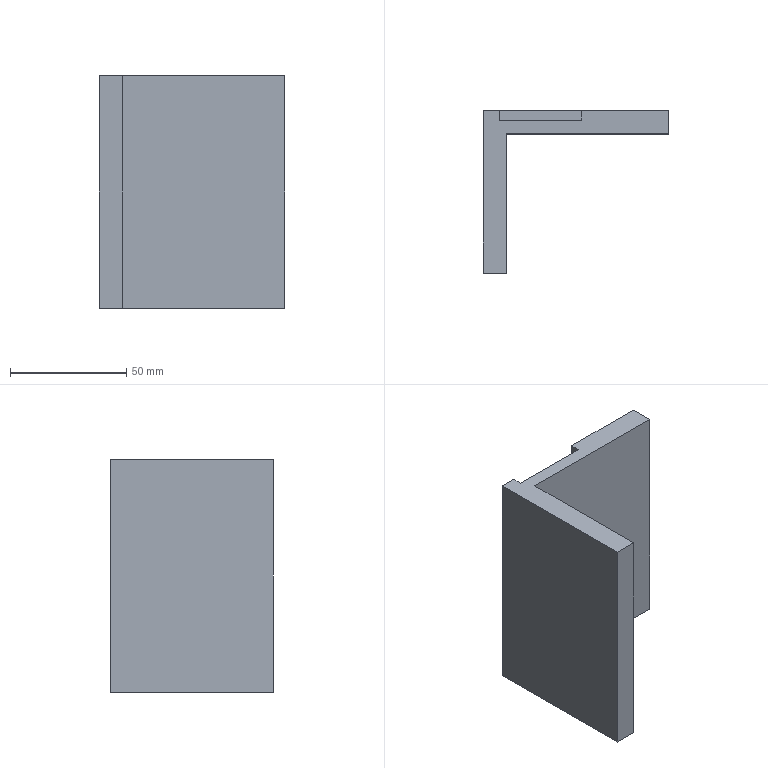Part | SolidWorks | features Cut 1, Extrusion 1 | 1 solid | 12 faces | box 80 x 70 x 100 mm | volume 131100 mm3 | plane 12
STEP:
#1=CARTESIAN_POINT('',(-37.5,32.788,0.));
#2=VERTEX_POINT('',#1);
#3=CARTESIAN_POINT('',(-37.5,-37.212,0.));
#4=VERTEX_POINT('',#3);
#5=CARTESIAN_POINT('',(-37.5,-37.212,0.));
#6=DIRECTION('',(0.,-1.,0.));
#7=VECTOR('',#6,1000.);
#8=LINE('',#5,#7);
#9=EDGE_CURVE('',#2,#4,#8,.T.);
#10=ORIENTED_EDGE('',*,*,#9,.T.);
#11=CARTESIAN_POINT('',(-37.5,-37.212,100.));
#12=VERTEX_POINT('',#11);
#13=CARTESIAN_POINT('',(-37.5,-37.212,100.));
#14=DIRECTION('',(0.,0.,-1.));
#15=VECTOR('',#14,1000.);
#16=LINE('',#13,#15);
#17=EDGE_CURVE('',#12,#4,#16,.T.);
#18=ORIENTED_EDGE('',*,*,#17,.F.);
#19=CARTESIAN_POINT('',(-37.5,32.788,100.));
#20=VERTEX_POINT('',#19);
#21=CARTESIAN_POINT('',(-37.5,-37.212,100.));
#22=DIRECTION('',(0.,-1.,0.));
#23=VECTOR('',#22,1000.);
#24=LINE('',#21,#23);
#25=EDGE_CURVE('',#20,#12,#24,.T.);
#26=ORIENTED_EDGE('',*,*,#25,.F.);
#27=CARTESIAN_POINT('',(-37.5,32.788,100.));
#28=DIRECTION('',(0.,0.,-1.));
#29=VECTOR('',#28,1000.);
#30=LINE('',#27,#29);
#31=EDGE_CURVE('',#20,#2,#30,.T.);
#32=ORIENTED_EDGE('',*,*,#31,.T.);
#33=EDGE_LOOP('',(#10,#18,#26,#32));
#34=FACE_OUTER_BOUND('',#33,.T.);
#35=CARTESIAN_POINT('',(-37.5,-37.212,100.));
#36=DIRECTION('',(1.,0.,0.));
#37=DIRECTION('',(0.,0.,-1.));
#38=AXIS2_PLACEMENT_3D('',#35,#36,#37);
#39=PLANE('',#38);
#40=ADVANCED_FACE('',(#34),#39,.F.);
#41=CARTESIAN_POINT('',(-27.5,-37.212,0.));
#42=VERTEX_POINT('',#41);
#43=CARTESIAN_POINT('',(-27.5,-37.212,0.));
#44=DIRECTION('',(1.,0.,0.));
#45=VECTOR('',#44,1000.);
#46=LINE('',#43,#45);
#47=EDGE_CURVE('',#4,#42,#46,.T.);
#48=ORIENTED_EDGE('',*,*,#47,.T.);
#49=CARTESIAN_POINT('',(-27.5,-37.212,100.));
#50=VERTEX_POINT('',#49);
#51=CARTESIAN_POINT('',(-27.5,-37.212,100.));
#52=DIRECTION('',(0.,0.,-1.));
#53=VECTOR('',#52,1000.);
#54=LINE('',#51,#53);
#55=EDGE_CURVE('',#50,#42,#54,.T.);
#56=ORIENTED_EDGE('',*,*,#55,.F.);
#57=CARTESIAN_POINT('',(-27.5,-37.212,100.));
#58=DIRECTION('',(1.,0.,0.));
#59=VECTOR('',#58,1000.);
#60=LINE('',#57,#59);
#61=EDGE_CURVE('',#12,#50,#60,.T.);
#62=ORIENTED_EDGE('',*,*,#61,.F.);
#63=ORIENTED_EDGE('',*,*,#17,.T.);
#64=EDGE_LOOP('',(#48,#56,#62,#63));
#65=FACE_OUTER_BOUND('',#64,.T.);
#66=CARTESIAN_POINT('',(-27.5,-37.212,100.));
#67=DIRECTION('',(0.,1.,0.));
#68=DIRECTION('',(0.,0.,1.));
#69=AXIS2_PLACEMENT_3D('',#66,#67,#68);
#70=PLANE('',#69);
#71=ADVANCED_FACE('',(#65),#70,.F.);
#72=CARTESIAN_POINT('',(-27.5,22.788,0.));
#73=VERTEX_POINT('',#72);
#74=CARTESIAN_POINT('',(-27.5,22.788,0.));
#75=DIRECTION('',(0.,1.,0.));
#76=VECTOR('',#75,1000.);
#77=LINE('',#74,#76);
#78=EDGE_CURVE('',#42,#73,#77,.T.);
#79=ORIENTED_EDGE('',*,*,#78,.T.);
#80=CARTESIAN_POINT('',(-27.5,22.788,100.));
#81=VERTEX_POINT('',#80);
#82=CARTESIAN_POINT('',(-27.5,22.788,100.));
#83=DIRECTION('',(0.,0.,-1.));
#84=VECTOR('',#83,1000.);
#85=LINE('',#82,#84);
#86=EDGE_CURVE('',#81,#73,#85,.T.);
#87=ORIENTED_EDGE('',*,*,#86,.F.);
#88=CARTESIAN_POINT('',(-27.5,22.788,100.));
#89=DIRECTION('',(0.,1.,0.));
#90=VECTOR('',#89,1000.);
#91=LINE('',#88,#90);
#92=EDGE_CURVE('',#50,#81,#91,.T.);
#93=ORIENTED_EDGE('',*,*,#92,.F.);
#94=ORIENTED_EDGE('',*,*,#55,.T.);
#95=EDGE_LOOP('',(#79,#87,#93,#94));
#96=FACE_OUTER_BOUND('',#95,.T.);
#97=CARTESIAN_POINT('',(-27.5,22.788,100.));
#98=DIRECTION('',(-1.,0.,0.));
#99=DIRECTION('',(0.,-1.,0.));
#100=AXIS2_PLACEMENT_3D('',#97,#98,#99);
#101=PLANE('',#100);
#102=ADVANCED_FACE('',(#96),#101,.F.);
#103=CARTESIAN_POINT('',(42.5,22.788,0.));
#104=VERTEX_POINT('',#103);
#105=CARTESIAN_POINT('',(42.5,22.788,0.));
#106=DIRECTION('',(1.,0.,0.));
#107=VECTOR('',#106,1000.);
#108=LINE('',#105,#107);
#109=EDGE_CURVE('',#73,#104,#108,.T.);
#110=ORIENTED_EDGE('',*,*,#109,.T.);
#111=CARTESIAN_POINT('',(42.5,22.788,100.));
#112=VERTEX_POINT('',#111);
#113=CARTESIAN_POINT('',(42.5,22.788,100.));
#114=DIRECTION('',(0.,0.,-1.));
#115=VECTOR('',#114,1000.);
#116=LINE('',#113,#115);
#117=EDGE_CURVE('',#112,#104,#116,.T.);
#118=ORIENTED_EDGE('',*,*,#117,.F.);
#119=CARTESIAN_POINT('',(42.5,22.788,100.));
#120=DIRECTION('',(1.,0.,0.));
#121=VECTOR('',#120,1000.);
#122=LINE('',#119,#121);
#123=EDGE_CURVE('',#81,#112,#122,.T.);
#124=ORIENTED_EDGE('',*,*,#123,.F.);
#125=ORIENTED_EDGE('',*,*,#86,.T.);
#126=EDGE_LOOP('',(#110,#118,#124,#125));
#127=FACE_OUTER_BOUND('',#126,.T.);
#128=CARTESIAN_POINT('',(42.5,22.788,100.));
#129=DIRECTION('',(0.,1.,0.));
#130=DIRECTION('',(-1.,0.,0.));
#131=AXIS2_PLACEMENT_3D('',#128,#129,#130);
#132=PLANE('',#131);
#133=ADVANCED_FACE('',(#127),#132,.F.);
#134=CARTESIAN_POINT('',(42.5,32.788,0.));
#135=VERTEX_POINT('',#134);
#136=CARTESIAN_POINT('',(42.5,32.788,0.));
#137=DIRECTION('',(0.,1.,0.));
#138=VECTOR('',#137,1000.);
#139=LINE('',#136,#138);
#140=EDGE_CURVE('',#104,#135,#139,.T.);
#141=ORIENTED_EDGE('',*,*,#140,.T.);
#142=CARTESIAN_POINT('',(42.5,32.788,100.));
#143=VERTEX_POINT('',#142);
#144=CARTESIAN_POINT('',(42.5,32.788,100.));
#145=DIRECTION('',(0.,0.,-1.));
#146=VECTOR('',#145,1000.);
#147=LINE('',#144,#146);
#148=EDGE_CURVE('',#143,#135,#147,.T.);
#149=ORIENTED_EDGE('',*,*,#148,.F.);
#150=CARTESIAN_POINT('',(42.5,32.788,100.));
#151=DIRECTION('',(0.,1.,0.));
#152=VECTOR('',#151,1000.);
#153=LINE('',#150,#152);
#154=EDGE_CURVE('',#112,#143,#153,.T.);
#155=ORIENTED_EDGE('',*,*,#154,.F.);
#156=ORIENTED_EDGE('',*,*,#117,.T.);
#157=EDGE_LOOP('',(#141,#149,#155,#156));
#158=FACE_OUTER_BOUND('',#157,.T.);
#159=CARTESIAN_POINT('',(42.5,32.788,100.));
#160=DIRECTION('',(-1.,0.,0.));
#161=DIRECTION('',(0.,0.,1.));
#162=AXIS2_PLACEMENT_3D('',#159,#160,#161);
#163=PLANE('',#162);
#164=ADVANCED_FACE('',(#158),#163,.F.);
#165=CARTESIAN_POINT('',(4.86,32.788,40.));
#166=VERTEX_POINT('',#165);
#167=CARTESIAN_POINT('',(-30.458,32.788,40.));
#168=VERTEX_POINT('',#167);
#169=CARTESIAN_POINT('',(4.86,32.788,40.));
#170=DIRECTION('',(-1.,0.,0.));
#171=VECTOR('',#170,1000.);
#172=LINE('',#169,#171);
#173=EDGE_CURVE('',#166,#168,#172,.T.);
#174=ORIENTED_EDGE('',*,*,#173,.F.);
#175=CARTESIAN_POINT('',(4.86,32.788,100.));
#176=VERTEX_POINT('',#175);
#177=CARTESIAN_POINT('',(4.86,32.788,40.));
#178=DIRECTION('',(0.,0.,1.));
#179=VECTOR('',#178,1000.);
#180=LINE('',#177,#179);
#181=EDGE_CURVE('',#166,#176,#180,.T.);
#182=ORIENTED_EDGE('',*,*,#181,.T.);
#183=CARTESIAN_POINT('',(-37.5,32.788,100.));
#184=DIRECTION('',(-1.,0.,0.));
#185=VECTOR('',#184,1000.);
#186=LINE('',#183,#185);
#187=EDGE_CURVE('',#143,#176,#186,.T.);
#188=ORIENTED_EDGE('',*,*,#187,.F.);
#189=ORIENTED_EDGE('',*,*,#148,.T.);
#190=CARTESIAN_POINT('',(-37.5,32.788,0.));
#191=DIRECTION('',(-1.,0.,0.));
#192=VECTOR('',#191,1000.);
#193=LINE('',#190,#192);
#194=EDGE_CURVE('',#135,#2,#193,.T.);
#195=ORIENTED_EDGE('',*,*,#194,.T.);
#196=ORIENTED_EDGE('',*,*,#31,.F.);
#197=CARTESIAN_POINT('',(-30.458,32.788,100.));
#198=VERTEX_POINT('',#197);
#199=CARTESIAN_POINT('',(-37.5,32.788,100.));
#200=DIRECTION('',(-1.,0.,0.));
#201=VECTOR('',#200,1000.);
#202=LINE('',#199,#201);
#203=EDGE_CURVE('',#198,#20,#202,.T.);
#204=ORIENTED_EDGE('',*,*,#203,.F.);
#205=CARTESIAN_POINT('',(-30.458,32.788,40.));
#206=DIRECTION('',(0.,0.,1.));
#207=VECTOR('',#206,1000.);
#208=LINE('',#205,#207);
#209=EDGE_CURVE('',#168,#198,#208,.T.);
#210=ORIENTED_EDGE('',*,*,#209,.F.);
#211=EDGE_LOOP('',(#174,#182,#188,#189,#195,#196,#204,#210));
#212=FACE_OUTER_BOUND('',#211,.T.);
#213=CARTESIAN_POINT('',(-37.5,32.788,100.));
#214=DIRECTION('',(0.,-1.,0.));
#215=DIRECTION('',(1.,0.,0.));
#216=AXIS2_PLACEMENT_3D('',#213,#214,#215);
#217=PLANE('',#216);
#218=ADVANCED_FACE('',(#212),#217,.F.);
#219=ORIENTED_EDGE('',*,*,#187,.T.);
#220=CARTESIAN_POINT('',(4.86,28.588,100.));
#221=VERTEX_POINT('',#220);
#222=CARTESIAN_POINT('',(4.86,28.588,100.));
#223=DIRECTION('',(0.,1.,0.));
#224=VECTOR('',#223,1000.);
#225=LINE('',#222,#224);
#226=EDGE_CURVE('',#221,#176,#225,.T.);
#227=ORIENTED_EDGE('',*,*,#226,.F.);
#228=CARTESIAN_POINT('',(-30.458,28.588,100.));
#229=VERTEX_POINT('',#228);
#230=CARTESIAN_POINT('',(-30.458,28.588,100.));
#231=DIRECTION('',(1.,0.,0.));
#232=VECTOR('',#231,1000.);
#233=LINE('',#230,#232);
#234=EDGE_CURVE('',#229,#221,#233,.T.);
#235=ORIENTED_EDGE('',*,*,#234,.F.);
#236=CARTESIAN_POINT('',(-30.458,32.788,100.));
#237=DIRECTION('',(0.,-1.,0.));
#238=VECTOR('',#237,1000.);
#239=LINE('',#236,#238);
#240=EDGE_CURVE('',#198,#229,#239,.T.);
#241=ORIENTED_EDGE('',*,*,#240,.F.);
#242=ORIENTED_EDGE('',*,*,#203,.T.);
#243=ORIENTED_EDGE('',*,*,#25,.T.);
#244=ORIENTED_EDGE('',*,*,#61,.T.);
#245=ORIENTED_EDGE('',*,*,#92,.T.);
#246=ORIENTED_EDGE('',*,*,#123,.T.);
#247=ORIENTED_EDGE('',*,*,#154,.T.);
#248=EDGE_LOOP('',(#219,#227,#235,#241,#242,#243,#244,#245,#246,#247));
#249=FACE_OUTER_BOUND('',#248,.T.);
#250=CARTESIAN_POINT('',(0.,0.,100.));
#251=DIRECTION('',(0.,0.,-1.));
#252=DIRECTION('',(-1.,0.,0.));
#253=AXIS2_PLACEMENT_3D('',#250,#251,#252);
#254=PLANE('',#253);
#255=ADVANCED_FACE('',(#249),#254,.F.);
#256=ORIENTED_EDGE('',*,*,#9,.F.);
#257=ORIENTED_EDGE('',*,*,#194,.F.);
#258=ORIENTED_EDGE('',*,*,#140,.F.);
#259=ORIENTED_EDGE('',*,*,#109,.F.);
#260=ORIENTED_EDGE('',*,*,#78,.F.);
#261=ORIENTED_EDGE('',*,*,#47,.F.);
#262=EDGE_LOOP('',(#256,#257,#258,#259,#260,#261));
#263=FACE_OUTER_BOUND('',#262,.T.);
#264=CARTESIAN_POINT('',(0.,0.,0.));
#265=DIRECTION('',(0.,0.,-1.));
#266=DIRECTION('',(-1.,0.,0.));
#267=AXIS2_PLACEMENT_3D('',#264,#265,#266);
#268=PLANE('',#267);
#269=ADVANCED_FACE('',(#263),#268,.T.);
#270=ORIENTED_EDGE('',*,*,#226,.T.);
#271=ORIENTED_EDGE('',*,*,#181,.F.);
#272=CARTESIAN_POINT('',(4.86,28.588,40.));
#273=VERTEX_POINT('',#272);
#274=CARTESIAN_POINT('',(4.86,28.588,40.));
#275=DIRECTION('',(0.,1.,0.));
#276=VECTOR('',#275,1000.);
#277=LINE('',#274,#276);
#278=EDGE_CURVE('',#273,#166,#277,.T.);
#279=ORIENTED_EDGE('',*,*,#278,.F.);
#280=CARTESIAN_POINT('',(4.86,28.588,40.));
#281=DIRECTION('',(0.,0.,1.));
#282=VECTOR('',#281,1000.);
#283=LINE('',#280,#282);
#284=EDGE_CURVE('',#273,#221,#283,.T.);
#285=ORIENTED_EDGE('',*,*,#284,.T.);
#286=EDGE_LOOP('',(#270,#271,#279,#285));
#287=FACE_OUTER_BOUND('',#286,.T.);
#288=CARTESIAN_POINT('',(4.86,28.588,40.));
#289=DIRECTION('',(1.,0.,0.));
#290=DIRECTION('',(0.,0.,-1.));
#291=AXIS2_PLACEMENT_3D('',#288,#289,#290);
#292=PLANE('',#291);
#293=ADVANCED_FACE('',(#287),#292,.F.);
#294=ORIENTED_EDGE('',*,*,#234,.T.);
#295=ORIENTED_EDGE('',*,*,#284,.F.);
#296=CARTESIAN_POINT('',(-30.458,28.588,40.));
#297=VERTEX_POINT('',#296);
#298=CARTESIAN_POINT('',(-30.458,28.588,40.));
#299=DIRECTION('',(1.,0.,0.));
#300=VECTOR('',#299,1000.);
#301=LINE('',#298,#300);
#302=EDGE_CURVE('',#297,#273,#301,.T.);
#303=ORIENTED_EDGE('',*,*,#302,.F.);
#304=CARTESIAN_POINT('',(-30.458,28.588,40.));
#305=DIRECTION('',(0.,0.,1.));
#306=VECTOR('',#305,1000.);
#307=LINE('',#304,#306);
#308=EDGE_CURVE('',#297,#229,#307,.T.);
#309=ORIENTED_EDGE('',*,*,#308,.T.);
#310=EDGE_LOOP('',(#294,#295,#303,#309));
#311=FACE_OUTER_BOUND('',#310,.T.);
#312=CARTESIAN_POINT('',(-30.458,28.588,40.));
#313=DIRECTION('',(0.,-1.,0.));
#314=DIRECTION('',(0.,0.,-1.));
#315=AXIS2_PLACEMENT_3D('',#312,#313,#314);
#316=PLANE('',#315);
#317=ADVANCED_FACE('',(#311),#316,.F.);
#318=ORIENTED_EDGE('',*,*,#240,.T.);
#319=ORIENTED_EDGE('',*,*,#308,.F.);
#320=CARTESIAN_POINT('',(-30.458,32.788,40.));
#321=DIRECTION('',(0.,-1.,0.));
#322=VECTOR('',#321,1000.);
#323=LINE('',#320,#322);
#324=EDGE_CURVE('',#168,#297,#323,.T.);
#325=ORIENTED_EDGE('',*,*,#324,.F.);
#326=ORIENTED_EDGE('',*,*,#209,.T.);
#327=EDGE_LOOP('',(#318,#319,#325,#326));
#328=FACE_OUTER_BOUND('',#327,.T.);
#329=CARTESIAN_POINT('',(-30.458,32.788,40.));
#330=DIRECTION('',(-1.,0.,0.));
#331=DIRECTION('',(0.,0.,1.));
#332=AXIS2_PLACEMENT_3D('',#329,#330,#331);
#333=PLANE('',#332);
#334=ADVANCED_FACE('',(#328),#333,.F.);
#335=ORIENTED_EDGE('',*,*,#173,.T.);
#336=ORIENTED_EDGE('',*,*,#324,.T.);
#337=ORIENTED_EDGE('',*,*,#302,.T.);
#338=ORIENTED_EDGE('',*,*,#278,.T.);
#339=EDGE_LOOP('',(#335,#336,#337,#338));
#340=FACE_OUTER_BOUND('',#339,.T.);
#341=CARTESIAN_POINT('',(0.,0.,40.));
#342=DIRECTION('',(0.,0.,1.));
#343=DIRECTION('',(1.,0.,0.));
#344=AXIS2_PLACEMENT_3D('',#341,#342,#343);
#345=PLANE('',#344);
#346=ADVANCED_FACE('',(#340),#345,.T.);
#347=CLOSED_SHELL('',(#40,#71,#102,#133,#164,#218,#255,#269,#293,#317,#334,#346));
#348=MANIFOLD_SOLID_BREP('',#347);
#349=CARTESIAN_POINT('',(0.,0.,0.));
#350=DIRECTION('',(0.,0.,1.));
#351=DIRECTION('',(1.,0.,0.));
#352=AXIS2_PLACEMENT_3D('',#349,#350,#351);
#353=(LENGTH_UNIT()NAMED_UNIT(*)SI_UNIT(.MILLI.,.METRE.));
#354=UNCERTAINTY_MEASURE_WITH_UNIT(LENGTH_MEASURE(0.00001),#353,'','');
#355=(NAMED_UNIT(*)PLANE_ANGLE_UNIT()SI_UNIT($,.RADIAN.));
#356=(NAMED_UNIT(*)SI_UNIT($,.STERADIAN.)SOLID_ANGLE_UNIT());
#357=(GEOMETRIC_REPRESENTATION_CONTEXT(3)GLOBAL_UNCERTAINTY_ASSIGNED_CONTEXT((#354))GLOBAL_UNIT_ASSIGNED_CONTEXT((#353,#355,#356))REPRESENTATION_CONTEXT('',''));
#358=ADVANCED_BREP_SHAPE_REPRESENTATION('',(#348,#352),#357);